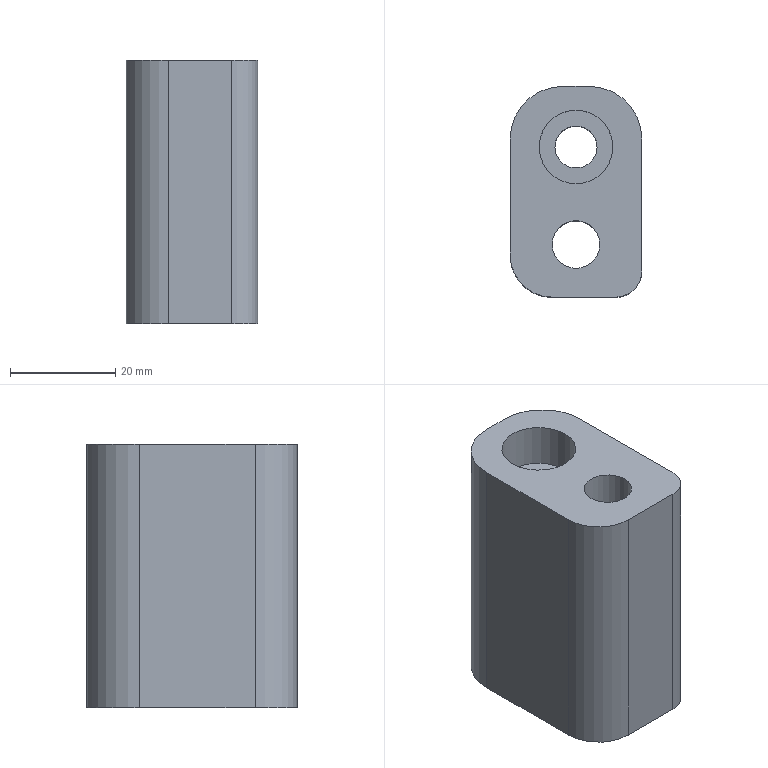Part | STEP file | PN_0014_id874_x_t | 1 solid | 16 faces | box 25 x 40 x 50 mm | volume 37635 mm3 | plane 8 | cylinder 8 | commonest cylinder face diameters 14 x2 20 x2 8 x1 9 x1 10 x1 16 x1
STEP:
#1=CARTESIAN_POINT('',(-238.,47.,95.));
#2=VERTEX_POINT('',#1);
#3=CARTESIAN_POINT('',(-245.,47.,95.));
#4=DIRECTION('',(0.,0.,-1.));
#5=DIRECTION('',(1.,0.,0.));
#6=AXIS2_PLACEMENT_3D('',#3,#4,#5);
#7=CIRCLE('',#6,7.);
#8=EDGE_CURVE('',#2,#2,#7,.T.);
#9=ORIENTED_EDGE('',*,*,#8,.T.);
#10=EDGE_LOOP('',(#9));
#11=FACE_BOUND('',#10,.T.);
#12=CARTESIAN_POINT('',(-240.5,28.5,95.));
#13=VERTEX_POINT('',#12);
#14=CARTESIAN_POINT('',(-245.,28.5,95.));
#15=DIRECTION('',(0.,0.,1.));
#16=DIRECTION('',(1.,0.,0.));
#17=AXIS2_PLACEMENT_3D('',#14,#15,#16);
#18=CIRCLE('',#17,4.5);
#19=EDGE_CURVE('',#13,#13,#18,.T.);
#20=ORIENTED_EDGE('',*,*,#19,.F.);
#21=EDGE_LOOP('',(#20));
#22=FACE_BOUND('',#21,.T.);
#23=CARTESIAN_POINT('',(-257.5,26.5,95.));
#24=VERTEX_POINT('',#23);
#25=CARTESIAN_POINT('',(-257.5,48.5,95.));
#26=VERTEX_POINT('',#25);
#27=CARTESIAN_POINT('',(-257.5,47.,95.));
#28=DIRECTION('',(0.,1.,0.));
#29=VECTOR('',#28,1.);
#30=LINE('',#27,#29);
#31=EDGE_CURVE('',#24,#26,#30,.T.);
#32=ORIENTED_EDGE('',*,*,#31,.F.);
#33=CARTESIAN_POINT('',(-249.5,18.5,95.));
#34=VERTEX_POINT('',#33);
#35=CARTESIAN_POINT('',(-249.5,26.5,95.));
#36=DIRECTION('',(0.,0.,1.));
#37=DIRECTION('',(1.,0.,0.));
#38=AXIS2_PLACEMENT_3D('',#35,#36,#37);
#39=CIRCLE('',#38,8.);
#40=EDGE_CURVE('',#24,#34,#39,.T.);
#41=ORIENTED_EDGE('',*,*,#40,.T.);
#42=CARTESIAN_POINT('',(-237.5,18.5,95.));
#43=VERTEX_POINT('',#42);
#44=CARTESIAN_POINT('',(-245.,18.5,95.));
#45=DIRECTION('',(-1.,0.,0.));
#46=VECTOR('',#45,1.);
#47=LINE('',#44,#46);
#48=EDGE_CURVE('',#43,#34,#47,.T.);
#49=ORIENTED_EDGE('',*,*,#48,.F.);
#50=CARTESIAN_POINT('',(-232.5,23.5,95.));
#51=VERTEX_POINT('',#50);
#52=CARTESIAN_POINT('',(-237.5,23.5,95.));
#53=DIRECTION('',(0.,0.,1.));
#54=DIRECTION('',(1.,0.,0.));
#55=AXIS2_PLACEMENT_3D('',#52,#53,#54);
#56=CIRCLE('',#55,5.);
#57=EDGE_CURVE('',#43,#51,#56,.T.);
#58=ORIENTED_EDGE('',*,*,#57,.T.);
#59=CARTESIAN_POINT('',(-232.5,48.5,95.));
#60=VERTEX_POINT('',#59);
#61=CARTESIAN_POINT('',(-232.5,47.,95.));
#62=DIRECTION('',(0.,-1.,0.));
#63=VECTOR('',#62,1.);
#64=LINE('',#61,#63);
#65=EDGE_CURVE('',#60,#51,#64,.T.);
#66=ORIENTED_EDGE('',*,*,#65,.F.);
#67=CARTESIAN_POINT('',(-242.5,58.5,95.));
#68=VERTEX_POINT('',#67);
#69=CARTESIAN_POINT('',(-242.5,48.5,95.));
#70=DIRECTION('',(0.,0.,1.));
#71=DIRECTION('',(1.,0.,0.));
#72=AXIS2_PLACEMENT_3D('',#69,#70,#71);
#73=CIRCLE('',#72,10.);
#74=EDGE_CURVE('',#60,#68,#73,.T.);
#75=ORIENTED_EDGE('',*,*,#74,.T.);
#76=CARTESIAN_POINT('',(-247.5,58.5,95.));
#77=VERTEX_POINT('',#76);
#78=CARTESIAN_POINT('',(-245.,58.5,95.));
#79=DIRECTION('',(1.,0.,0.));
#80=VECTOR('',#79,1.);
#81=LINE('',#78,#80);
#82=EDGE_CURVE('',#77,#68,#81,.T.);
#83=ORIENTED_EDGE('',*,*,#82,.F.);
#84=CARTESIAN_POINT('',(-247.5,48.5,95.));
#85=DIRECTION('',(0.,0.,1.));
#86=DIRECTION('',(1.,0.,0.));
#87=AXIS2_PLACEMENT_3D('',#84,#85,#86);
#88=CIRCLE('',#87,10.);
#89=EDGE_CURVE('',#77,#26,#88,.T.);
#90=ORIENTED_EDGE('',*,*,#89,.T.);
#91=EDGE_LOOP('',(#32,#41,#49,#58,#66,#75,#83,#90));
#92=FACE_BOUND('',#91,.T.);
#93=CARTESIAN_POINT('',(-245.,47.,95.));
#94=DIRECTION('',(0.,0.,1.));
#95=DIRECTION('',(1.,0.,0.));
#96=AXIS2_PLACEMENT_3D('',#93,#94,#95);
#97=PLANE('',#96);
#98=ADVANCED_FACE('',(#11,#22,#92),#97,.T.);
#99=ORIENTED_EDGE('',*,*,#48,.T.);
#100=CARTESIAN_POINT('',(-249.5,18.5,45.));
#101=VERTEX_POINT('',#100);
#102=CARTESIAN_POINT('',(-249.5,18.5,5.));
#103=DIRECTION('',(0.,0.,-1.));
#104=VECTOR('',#103,1.);
#105=LINE('',#102,#104);
#106=EDGE_CURVE('',#34,#101,#105,.T.);
#107=ORIENTED_EDGE('',*,*,#106,.T.);
#108=CARTESIAN_POINT('',(-237.5,18.5,45.));
#109=VERTEX_POINT('',#108);
#110=CARTESIAN_POINT('',(-245.,18.5,45.));
#111=DIRECTION('',(1.,0.,0.));
#112=VECTOR('',#111,1.);
#113=LINE('',#110,#112);
#114=EDGE_CURVE('',#101,#109,#113,.T.);
#115=ORIENTED_EDGE('',*,*,#114,.T.);
#116=CARTESIAN_POINT('',(-237.5,18.5,5.));
#117=DIRECTION('',(0.,0.,1.));
#118=VECTOR('',#117,1.);
#119=LINE('',#116,#118);
#120=EDGE_CURVE('',#109,#43,#119,.T.);
#121=ORIENTED_EDGE('',*,*,#120,.T.);
#122=EDGE_LOOP('',(#99,#107,#115,#121));
#123=FACE_OUTER_BOUND('',#122,.T.);
#124=CARTESIAN_POINT('',(-245.,18.5,5.));
#125=DIRECTION('',(0.,-1.,0.));
#126=DIRECTION('',(0.,0.,-1.));
#127=AXIS2_PLACEMENT_3D('',#124,#125,#126);
#128=PLANE('',#127);
#129=ADVANCED_FACE('',(#123),#128,.T.);
#130=CARTESIAN_POINT('',(-257.5,48.5,45.));
#131=VERTEX_POINT('',#130);
#132=CARTESIAN_POINT('',(-257.5,26.5,45.));
#133=VERTEX_POINT('',#132);
#134=CARTESIAN_POINT('',(-257.5,47.,45.));
#135=DIRECTION('',(0.,-1.,0.));
#136=VECTOR('',#135,1.);
#137=LINE('',#134,#136);
#138=EDGE_CURVE('',#131,#133,#137,.T.);
#139=ORIENTED_EDGE('',*,*,#138,.T.);
#140=CARTESIAN_POINT('',(-257.5,26.5,5.));
#141=DIRECTION('',(0.,0.,1.));
#142=VECTOR('',#141,1.);
#143=LINE('',#140,#142);
#144=EDGE_CURVE('',#133,#24,#143,.T.);
#145=ORIENTED_EDGE('',*,*,#144,.T.);
#146=ORIENTED_EDGE('',*,*,#31,.T.);
#147=CARTESIAN_POINT('',(-257.5,48.5,5.));
#148=DIRECTION('',(0.,0.,-1.));
#149=VECTOR('',#148,1.);
#150=LINE('',#147,#149);
#151=EDGE_CURVE('',#26,#131,#150,.T.);
#152=ORIENTED_EDGE('',*,*,#151,.T.);
#153=EDGE_LOOP('',(#139,#145,#146,#152));
#154=FACE_OUTER_BOUND('',#153,.T.);
#155=CARTESIAN_POINT('',(-257.5,47.,5.));
#156=DIRECTION('',(-1.,0.,0.));
#157=DIRECTION('',(0.,0.,1.));
#158=AXIS2_PLACEMENT_3D('',#155,#156,#157);
#159=PLANE('',#158);
#160=ADVANCED_FACE('',(#154),#159,.T.);
#161=ORIENTED_EDGE('',*,*,#82,.T.);
#162=CARTESIAN_POINT('',(-242.5,58.5,45.));
#163=VERTEX_POINT('',#162);
#164=CARTESIAN_POINT('',(-242.5,58.5,5.));
#165=DIRECTION('',(0.,0.,-1.));
#166=VECTOR('',#165,1.);
#167=LINE('',#164,#166);
#168=EDGE_CURVE('',#68,#163,#167,.T.);
#169=ORIENTED_EDGE('',*,*,#168,.T.);
#170=CARTESIAN_POINT('',(-247.5,58.5,45.));
#171=VERTEX_POINT('',#170);
#172=CARTESIAN_POINT('',(-245.,58.5,45.));
#173=DIRECTION('',(-1.,0.,0.));
#174=VECTOR('',#173,1.);
#175=LINE('',#172,#174);
#176=EDGE_CURVE('',#163,#171,#175,.T.);
#177=ORIENTED_EDGE('',*,*,#176,.T.);
#178=CARTESIAN_POINT('',(-247.5,58.5,5.));
#179=DIRECTION('',(0.,0.,1.));
#180=VECTOR('',#179,1.);
#181=LINE('',#178,#180);
#182=EDGE_CURVE('',#171,#77,#181,.T.);
#183=ORIENTED_EDGE('',*,*,#182,.T.);
#184=EDGE_LOOP('',(#161,#169,#177,#183));
#185=FACE_OUTER_BOUND('',#184,.T.);
#186=CARTESIAN_POINT('',(-245.,58.5,5.));
#187=DIRECTION('',(0.,1.,0.));
#188=DIRECTION('',(0.,0.,1.));
#189=AXIS2_PLACEMENT_3D('',#186,#187,#188);
#190=PLANE('',#189);
#191=ADVANCED_FACE('',(#185),#190,.T.);
#192=CARTESIAN_POINT('',(-241.,47.,45.));
#193=VERTEX_POINT('',#192);
#194=CARTESIAN_POINT('',(-245.,47.,45.));
#195=DIRECTION('',(0.,0.,1.));
#196=DIRECTION('',(1.,0.,0.));
#197=AXIS2_PLACEMENT_3D('',#194,#195,#196);
#198=CIRCLE('',#197,4.);
#199=EDGE_CURVE('',#193,#193,#198,.T.);
#200=ORIENTED_EDGE('',*,*,#199,.T.);
#201=EDGE_LOOP('',(#200));
#202=FACE_BOUND('',#201,.T.);
#203=CARTESIAN_POINT('',(-238.,28.5,45.));
#204=VERTEX_POINT('',#203);
#205=CARTESIAN_POINT('',(-245.,28.5,45.));
#206=DIRECTION('',(0.,0.,1.));
#207=DIRECTION('',(1.,0.,0.));
#208=AXIS2_PLACEMENT_3D('',#205,#206,#207);
#209=CIRCLE('',#208,7.);
#210=EDGE_CURVE('',#204,#204,#209,.T.);
#211=ORIENTED_EDGE('',*,*,#210,.T.);
#212=EDGE_LOOP('',(#211));
#213=FACE_BOUND('',#212,.T.);
#214=ORIENTED_EDGE('',*,*,#114,.F.);
#215=CARTESIAN_POINT('',(-249.5,26.5,45.));
#216=DIRECTION('',(0.,0.,-1.));
#217=DIRECTION('',(1.,0.,0.));
#218=AXIS2_PLACEMENT_3D('',#215,#216,#217);
#219=CIRCLE('',#218,8.);
#220=EDGE_CURVE('',#101,#133,#219,.T.);
#221=ORIENTED_EDGE('',*,*,#220,.T.);
#222=ORIENTED_EDGE('',*,*,#138,.F.);
#223=CARTESIAN_POINT('',(-247.5,48.5,45.));
#224=DIRECTION('',(0.,0.,-1.));
#225=DIRECTION('',(1.,0.,0.));
#226=AXIS2_PLACEMENT_3D('',#223,#224,#225);
#227=CIRCLE('',#226,10.);
#228=EDGE_CURVE('',#131,#171,#227,.T.);
#229=ORIENTED_EDGE('',*,*,#228,.T.);
#230=ORIENTED_EDGE('',*,*,#176,.F.);
#231=CARTESIAN_POINT('',(-232.5,48.5,45.));
#232=VERTEX_POINT('',#231);
#233=CARTESIAN_POINT('',(-242.5,48.5,45.));
#234=DIRECTION('',(0.,0.,-1.));
#235=DIRECTION('',(1.,0.,0.));
#236=AXIS2_PLACEMENT_3D('',#233,#234,#235);
#237=CIRCLE('',#236,10.);
#238=EDGE_CURVE('',#163,#232,#237,.T.);
#239=ORIENTED_EDGE('',*,*,#238,.T.);
#240=CARTESIAN_POINT('',(-232.5,23.5,45.));
#241=VERTEX_POINT('',#240);
#242=CARTESIAN_POINT('',(-232.5,47.,45.));
#243=DIRECTION('',(0.,1.,0.));
#244=VECTOR('',#243,1.);
#245=LINE('',#242,#244);
#246=EDGE_CURVE('',#241,#232,#245,.T.);
#247=ORIENTED_EDGE('',*,*,#246,.F.);
#248=CARTESIAN_POINT('',(-237.5,23.5,45.));
#249=DIRECTION('',(0.,0.,-1.));
#250=DIRECTION('',(1.,0.,0.));
#251=AXIS2_PLACEMENT_3D('',#248,#249,#250);
#252=CIRCLE('',#251,5.);
#253=EDGE_CURVE('',#241,#109,#252,.T.);
#254=ORIENTED_EDGE('',*,*,#253,.T.);
#255=EDGE_LOOP('',(#214,#221,#222,#229,#230,#239,#247,#254));
#256=FACE_BOUND('',#255,.T.);
#257=CARTESIAN_POINT('',(-119.811,64.,45.));
#258=DIRECTION('',(0.,0.,1.));
#259=DIRECTION('',(1.,0.,0.));
#260=AXIS2_PLACEMENT_3D('',#257,#258,#259);
#261=PLANE('',#260);
#262=ADVANCED_FACE('',(#202,#213,#256),#261,.F.);
#263=ORIENTED_EDGE('',*,*,#65,.T.);
#264=CARTESIAN_POINT('',(-232.5,23.5,5.));
#265=DIRECTION('',(0.,0.,-1.));
#266=VECTOR('',#265,1.);
#267=LINE('',#264,#266);
#268=EDGE_CURVE('',#51,#241,#267,.T.);
#269=ORIENTED_EDGE('',*,*,#268,.T.);
#270=ORIENTED_EDGE('',*,*,#246,.T.);
#271=CARTESIAN_POINT('',(-232.5,48.5,5.));
#272=DIRECTION('',(0.,0.,1.));
#273=VECTOR('',#272,1.);
#274=LINE('',#271,#273);
#275=EDGE_CURVE('',#232,#60,#274,.T.);
#276=ORIENTED_EDGE('',*,*,#275,.T.);
#277=EDGE_LOOP('',(#263,#269,#270,#276));
#278=FACE_OUTER_BOUND('',#277,.T.);
#279=CARTESIAN_POINT('',(-232.5,47.,5.));
#280=DIRECTION('',(1.,0.,0.));
#281=DIRECTION('',(0.,0.,-1.));
#282=AXIS2_PLACEMENT_3D('',#279,#280,#281);
#283=PLANE('',#282);
#284=ADVANCED_FACE('',(#278),#283,.T.);
#285=ORIENTED_EDGE('',*,*,#238,.F.);
#286=ORIENTED_EDGE('',*,*,#168,.F.);
#287=ORIENTED_EDGE('',*,*,#74,.F.);
#288=ORIENTED_EDGE('',*,*,#275,.F.);
#289=EDGE_LOOP('',(#285,#286,#287,#288));
#290=FACE_OUTER_BOUND('',#289,.T.);
#291=CARTESIAN_POINT('',(-242.5,48.5,5.));
#292=DIRECTION('',(0.,0.,1.));
#293=DIRECTION('',(1.,0.,0.));
#294=AXIS2_PLACEMENT_3D('',#291,#292,#293);
#295=CYLINDRICAL_SURFACE('',#294,10.);
#296=ADVANCED_FACE('',(#290),#295,.T.);
#297=ORIENTED_EDGE('',*,*,#228,.F.);
#298=ORIENTED_EDGE('',*,*,#151,.F.);
#299=ORIENTED_EDGE('',*,*,#89,.F.);
#300=ORIENTED_EDGE('',*,*,#182,.F.);
#301=EDGE_LOOP('',(#297,#298,#299,#300));
#302=FACE_OUTER_BOUND('',#301,.T.);
#303=CARTESIAN_POINT('',(-247.5,48.5,5.));
#304=DIRECTION('',(0.,0.,1.));
#305=DIRECTION('',(1.,0.,0.));
#306=AXIS2_PLACEMENT_3D('',#303,#304,#305);
#307=CYLINDRICAL_SURFACE('',#306,10.);
#308=ADVANCED_FACE('',(#302),#307,.T.);
#309=ORIENTED_EDGE('',*,*,#253,.F.);
#310=ORIENTED_EDGE('',*,*,#268,.F.);
#311=ORIENTED_EDGE('',*,*,#57,.F.);
#312=ORIENTED_EDGE('',*,*,#120,.F.);
#313=EDGE_LOOP('',(#309,#310,#311,#312));
#314=FACE_OUTER_BOUND('',#313,.T.);
#315=CARTESIAN_POINT('',(-237.5,23.5,5.));
#316=DIRECTION('',(0.,0.,1.));
#317=DIRECTION('',(1.,0.,0.));
#318=AXIS2_PLACEMENT_3D('',#315,#316,#317);
#319=CYLINDRICAL_SURFACE('',#318,5.);
#320=ADVANCED_FACE('',(#314),#319,.T.);
#321=ORIENTED_EDGE('',*,*,#220,.F.);
#322=ORIENTED_EDGE('',*,*,#106,.F.);
#323=ORIENTED_EDGE('',*,*,#40,.F.);
#324=ORIENTED_EDGE('',*,*,#144,.F.);
#325=EDGE_LOOP('',(#321,#322,#323,#324));
#326=FACE_OUTER_BOUND('',#325,.T.);
#327=CARTESIAN_POINT('',(-249.5,26.5,5.));
#328=DIRECTION('',(0.,0.,1.));
#329=DIRECTION('',(1.,0.,0.));
#330=AXIS2_PLACEMENT_3D('',#327,#328,#329);
#331=CYLINDRICAL_SURFACE('',#330,8.);
#332=ADVANCED_FACE('',(#326),#331,.T.);
#333=ORIENTED_EDGE('',*,*,#19,.T.);
#334=EDGE_LOOP('',(#333));
#335=FACE_BOUND('',#334,.T.);
#336=CARTESIAN_POINT('',(-240.5,28.5,75.));
#337=VERTEX_POINT('',#336);
#338=CARTESIAN_POINT('',(-245.,28.5,75.));
#339=DIRECTION('',(0.,0.,1.));
#340=DIRECTION('',(1.,0.,0.));
#341=AXIS2_PLACEMENT_3D('',#338,#339,#340);
#342=CIRCLE('',#341,4.5);
#343=EDGE_CURVE('',#337,#337,#342,.T.);
#344=ORIENTED_EDGE('',*,*,#343,.F.);
#345=EDGE_LOOP('',(#344));
#346=FACE_BOUND('',#345,.T.);
#347=CARTESIAN_POINT('',(-245.,28.5,105.));
#348=DIRECTION('',(0.,0.,-1.));
#349=DIRECTION('',(-1.,0.,0.));
#350=AXIS2_PLACEMENT_3D('',#347,#348,#349);
#351=CYLINDRICAL_SURFACE('',#350,4.5);
#352=ADVANCED_FACE('',(#335,#346),#351,.F.);
#353=ORIENTED_EDGE('',*,*,#343,.T.);
#354=EDGE_LOOP('',(#353));
#355=FACE_BOUND('',#354,.T.);
#356=CARTESIAN_POINT('',(-252.,28.5,75.));
#357=VERTEX_POINT('',#356);
#358=CARTESIAN_POINT('',(-245.,28.5,75.));
#359=DIRECTION('',(0.,0.,1.));
#360=DIRECTION('',(-1.,0.,0.));
#361=AXIS2_PLACEMENT_3D('',#358,#359,#360);
#362=CIRCLE('',#361,7.);
#363=EDGE_CURVE('',#357,#357,#362,.T.);
#364=ORIENTED_EDGE('',*,*,#363,.F.);
#365=EDGE_LOOP('',(#364));
#366=FACE_BOUND('',#365,.T.);
#367=CARTESIAN_POINT('',(-245.,28.5,75.));
#368=DIRECTION('',(0.,0.,1.));
#369=DIRECTION('',(1.,0.,0.));
#370=AXIS2_PLACEMENT_3D('',#367,#368,#369);
#371=PLANE('',#370);
#372=ADVANCED_FACE('',(#355,#366),#371,.F.);
#373=ORIENTED_EDGE('',*,*,#210,.F.);
#374=EDGE_LOOP('',(#373));
#375=FACE_BOUND('',#374,.T.);
#376=ORIENTED_EDGE('',*,*,#363,.T.);
#377=EDGE_LOOP('',(#376));
#378=FACE_BOUND('',#377,.T.);
#379=CARTESIAN_POINT('',(-245.,28.5,75.));
#380=DIRECTION('',(0.,0.,-1.));
#381=DIRECTION('',(-1.,0.,0.));
#382=AXIS2_PLACEMENT_3D('',#379,#380,#381);
#383=CYLINDRICAL_SURFACE('',#382,7.);
#384=ADVANCED_FACE('',(#375,#378),#383,.F.);
#385=CARTESIAN_POINT('',(-249.,47.,86.7));
#386=VERTEX_POINT('',#385);
#387=CARTESIAN_POINT('',(-245.,47.,86.7));
#388=DIRECTION('',(0.,0.,-1.));
#389=DIRECTION('',(-1.,0.,0.));
#390=AXIS2_PLACEMENT_3D('',#387,#388,#389);
#391=CIRCLE('',#390,4.);
#392=EDGE_CURVE('',#386,#386,#391,.T.);
#393=ORIENTED_EDGE('',*,*,#392,.F.);
#394=EDGE_LOOP('',(#393));
#395=FACE_BOUND('',#394,.T.);
#396=ORIENTED_EDGE('',*,*,#199,.F.);
#397=EDGE_LOOP('',(#396));
#398=FACE_BOUND('',#397,.T.);
#399=CARTESIAN_POINT('',(-245.,47.,85.5));
#400=DIRECTION('',(0.,0.,-1.));
#401=DIRECTION('',(0.,-1.,0.));
#402=AXIS2_PLACEMENT_3D('',#399,#400,#401);
#403=CYLINDRICAL_SURFACE('',#402,4.);
#404=ADVANCED_FACE('',(#395,#398),#403,.F.);
#405=ORIENTED_EDGE('',*,*,#392,.T.);
#406=EDGE_LOOP('',(#405));
#407=FACE_BOUND('',#406,.T.);
#408=CARTESIAN_POINT('',(-252.,47.,86.7));
#409=VERTEX_POINT('',#408);
#410=CARTESIAN_POINT('',(-245.,47.,86.7));
#411=DIRECTION('',(0.,0.,-1.));
#412=DIRECTION('',(-1.,0.,0.));
#413=AXIS2_PLACEMENT_3D('',#410,#411,#412);
#414=CIRCLE('',#413,7.);
#415=EDGE_CURVE('',#409,#409,#414,.T.);
#416=ORIENTED_EDGE('',*,*,#415,.F.);
#417=EDGE_LOOP('',(#416));
#418=FACE_BOUND('',#417,.T.);
#419=CARTESIAN_POINT('',(-245.,47.,86.7));
#420=DIRECTION('',(0.,0.,-1.));
#421=DIRECTION('',(-1.,0.,0.));
#422=AXIS2_PLACEMENT_3D('',#419,#420,#421);
#423=PLANE('',#422);
#424=ADVANCED_FACE('',(#407,#418),#423,.F.);
#425=ORIENTED_EDGE('',*,*,#415,.T.);
#426=EDGE_LOOP('',(#425));
#427=FACE_BOUND('',#426,.T.);
#428=ORIENTED_EDGE('',*,*,#8,.F.);
#429=EDGE_LOOP('',(#428));
#430=FACE_BOUND('',#429,.T.);
#431=CARTESIAN_POINT('',(-245.,47.,94.559));
#432=DIRECTION('',(0.,0.,-1.));
#433=DIRECTION('',(0.,-1.,0.));
#434=AXIS2_PLACEMENT_3D('',#431,#432,#433);
#435=CYLINDRICAL_SURFACE('',#434,7.);
#436=ADVANCED_FACE('',(#427,#430),#435,.F.);
#437=CLOSED_SHELL('',(#98,#129,#160,#191,#262,#284,#296,#308,#320,#332,#352,#372,#384,#404,#424,#436));
#438=MANIFOLD_SOLID_BREP('',#437);
#439=(LENGTH_UNIT()NAMED_UNIT(*)SI_UNIT(.MILLI.,.METRE.));
#440=UNCERTAINTY_MEASURE_WITH_UNIT(LENGTH_MEASURE(0.00002),#439,'','');
#441=(NAMED_UNIT(*)PLANE_ANGLE_UNIT()SI_UNIT($,.RADIAN.));
#442=PLANE_ANGLE_MEASURE_WITH_UNIT(PLANE_ANGLE_MEASURE(0.01745),#441);
#443=DIMENSIONAL_EXPONENTS(0.,0.,0.,0.,0.,0.,0.);
#444=(CONVERSION_BASED_UNIT('DEGREE',#442)NAMED_UNIT(#443)PLANE_ANGLE_UNIT());
#445=(NAMED_UNIT(*)SI_UNIT($,.STERADIAN.)SOLID_ANGLE_UNIT());
#446=(GEOMETRIC_REPRESENTATION_CONTEXT(3)GLOBAL_UNCERTAINTY_ASSIGNED_CONTEXT((#440))GLOBAL_UNIT_ASSIGNED_CONTEXT((#439,#444,#445))REPRESENTATION_CONTEXT('',''));
#447=ADVANCED_BREP_SHAPE_REPRESENTATION('',(#438),#446);